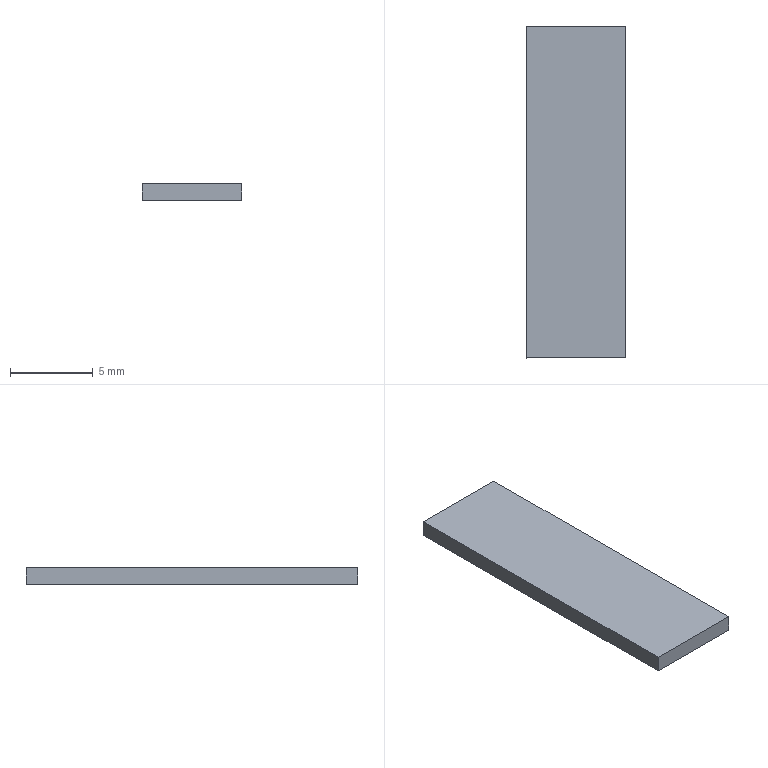Part | STEP file | RJ-USIO-V1_2-220411_235 | 1 solid | 6 faces | box 6 x 20.001 x 1 mm | volume 120.006 mm3 | plane 6
STEP:
#1=CARTESIAN_POINT('',(0.,0.,0.));
#2=DIRECTION('',(0.,0.,1.));
#3=DIRECTION('',(1.,0.,0.));
#4=AXIS2_PLACEMENT_3D('',#1,#2,#3);
#5=CARTESIAN_POINT('',(0.2,60.501,1.));
#6=VERTEX_POINT('',#5);
#7=CARTESIAN_POINT('',(0.2,40.5,1.));
#8=VERTEX_POINT('',#7);
#9=CARTESIAN_POINT('',(0.2,60.501,1.));
#10=DIRECTION('',(0.000000044,-1.,0.));
#11=VECTOR('',#10,1.);
#12=LINE('',#9,#11);
#13=CARTESIAN_POINT('',(0.2,40.5,1.));
#14=DIRECTION('',(0.,0.,-1.));
#15=DIRECTION('',(-0.000000044,1.,0.));
#16=AXIS2_PLACEMENT_3D('',#13,#14,#15);
#17=PLANE('',#16);
#18=CARTESIAN_POINT('',(20.001,0.));
#19=DIRECTION('',(-1.,0.));
#20=VECTOR('',#19,1.);
#21=LINE('',#18,#20);
#22=(GEOMETRIC_REPRESENTATION_CONTEXT(2)PARAMETRIC_REPRESENTATION_CONTEXT()REPRESENTATION_CONTEXT('',''));
#23=DEFINITIONAL_REPRESENTATION('',(#21),#22);
#24=PCURVE('',#17,#23);
#25=CARTESIAN_POINT('',(0.2,40.5,0.));
#26=DIRECTION('',(-1.,-0.000000044,0.));
#27=DIRECTION('',(0.000000044,-1.,0.));
#28=AXIS2_PLACEMENT_3D('',#25,#26,#27);
#29=PLANE('',#28);
#30=CARTESIAN_POINT('',(-20.001,1.));
#31=DIRECTION('',(1.,0.));
#32=VECTOR('',#31,1.);
#33=LINE('',#30,#32);
#34=(GEOMETRIC_REPRESENTATION_CONTEXT(2)PARAMETRIC_REPRESENTATION_CONTEXT()REPRESENTATION_CONTEXT('',''));
#35=DEFINITIONAL_REPRESENTATION('',(#33),#34);
#36=PCURVE('',#29,#35);
#37=SURFACE_CURVE('',#12,(#24,#36),.PCURVE_S1.);
#38=EDGE_CURVE('',#6,#8,#37,.T.);
#39=ORIENTED_EDGE('',*,*,#38,.T.);
#40=CARTESIAN_POINT('',(-5.8,40.5,1.));
#41=VERTEX_POINT('',#40);
#42=CARTESIAN_POINT('',(0.2,40.5,1.));
#43=DIRECTION('',(-1.,-0.000000044,0.));
#44=VECTOR('',#43,1.);
#45=LINE('',#42,#44);
#46=CARTESIAN_POINT('',(0.,0.));
#47=DIRECTION('',(0.,-1.));
#48=VECTOR('',#47,1.);
#49=LINE('',#46,#48);
#50=(GEOMETRIC_REPRESENTATION_CONTEXT(2)PARAMETRIC_REPRESENTATION_CONTEXT()REPRESENTATION_CONTEXT('',''));
#51=DEFINITIONAL_REPRESENTATION('',(#49),#50);
#52=PCURVE('',#17,#51);
#53=CARTESIAN_POINT('',(-5.8,40.5,0.));
#54=DIRECTION('',(-0.000000044,1.,0.));
#55=DIRECTION('',(-1.,-0.000000044,0.));
#56=AXIS2_PLACEMENT_3D('',#53,#54,#55);
#57=PLANE('',#56);
#58=CARTESIAN_POINT('',(-6.,1.));
#59=DIRECTION('',(1.,0.));
#60=VECTOR('',#59,1.);
#61=LINE('',#58,#60);
#62=(GEOMETRIC_REPRESENTATION_CONTEXT(2)PARAMETRIC_REPRESENTATION_CONTEXT()REPRESENTATION_CONTEXT('',''));
#63=DEFINITIONAL_REPRESENTATION('',(#61),#62);
#64=PCURVE('',#57,#63);
#65=SURFACE_CURVE('',#45,(#52,#64),.PCURVE_S1.);
#66=EDGE_CURVE('',#8,#41,#65,.T.);
#67=ORIENTED_EDGE('',*,*,#66,.T.);
#68=CARTESIAN_POINT('',(-5.8,60.501,1.));
#69=VERTEX_POINT('',#68);
#70=CARTESIAN_POINT('',(-5.8,40.5,1.));
#71=DIRECTION('',(-0.000000044,1.,0.));
#72=VECTOR('',#71,1.);
#73=LINE('',#70,#72);
#74=CARTESIAN_POINT('',(0.,-6.));
#75=DIRECTION('',(1.,0.));
#76=VECTOR('',#75,1.);
#77=LINE('',#74,#76);
#78=(GEOMETRIC_REPRESENTATION_CONTEXT(2)PARAMETRIC_REPRESENTATION_CONTEXT()REPRESENTATION_CONTEXT('',''));
#79=DEFINITIONAL_REPRESENTATION('',(#77),#78);
#80=PCURVE('',#17,#79);
#81=CARTESIAN_POINT('',(-5.8,60.5,0.));
#82=DIRECTION('',(1.,0.000000044,0.));
#83=DIRECTION('',(-0.000000044,1.,0.));
#84=AXIS2_PLACEMENT_3D('',#81,#82,#83);
#85=PLANE('',#84);
#86=CARTESIAN_POINT('',(-20.,1.));
#87=DIRECTION('',(1.,0.));
#88=VECTOR('',#87,1.);
#89=LINE('',#86,#88);
#90=(GEOMETRIC_REPRESENTATION_CONTEXT(2)PARAMETRIC_REPRESENTATION_CONTEXT()REPRESENTATION_CONTEXT('',''));
#91=DEFINITIONAL_REPRESENTATION('',(#89),#90);
#92=PCURVE('',#85,#91);
#93=SURFACE_CURVE('',#73,(#80,#92),.PCURVE_S1.);
#94=EDGE_CURVE('',#41,#69,#93,.T.);
#95=ORIENTED_EDGE('',*,*,#94,.T.);
#96=CARTESIAN_POINT('',(-5.8,60.501,1.));
#97=DIRECTION('',(1.,0.000000044,0.));
#98=VECTOR('',#97,1.);
#99=LINE('',#96,#98);
#100=CARTESIAN_POINT('',(20.001,-6.));
#101=DIRECTION('',(0.,1.));
#102=VECTOR('',#101,1.);
#103=LINE('',#100,#102);
#104=(GEOMETRIC_REPRESENTATION_CONTEXT(2)PARAMETRIC_REPRESENTATION_CONTEXT()REPRESENTATION_CONTEXT('',''));
#105=DEFINITIONAL_REPRESENTATION('',(#103),#104);
#106=PCURVE('',#17,#105);
#107=CARTESIAN_POINT('',(0.2,60.501,0.));
#108=DIRECTION('',(0.000000044,-1.,0.));
#109=DIRECTION('',(1.,0.000000044,0.));
#110=AXIS2_PLACEMENT_3D('',#107,#108,#109);
#111=PLANE('',#110);
#112=CARTESIAN_POINT('',(-6.,1.));
#113=DIRECTION('',(1.,0.));
#114=VECTOR('',#113,1.);
#115=LINE('',#112,#114);
#116=(GEOMETRIC_REPRESENTATION_CONTEXT(2)PARAMETRIC_REPRESENTATION_CONTEXT()REPRESENTATION_CONTEXT('',''));
#117=DEFINITIONAL_REPRESENTATION('',(#115),#116);
#118=PCURVE('',#111,#117);
#119=SURFACE_CURVE('',#99,(#106,#118),.PCURVE_S1.);
#120=EDGE_CURVE('',#69,#6,#119,.T.);
#121=ORIENTED_EDGE('',*,*,#120,.T.);
#122=EDGE_LOOP('',(#39,#67,#95,#121));
#123=FACE_BOUND('',#122,.F.);
#124=ADVANCED_FACE('',(#123),#17,.F.);
#125=CARTESIAN_POINT('',(0.2,60.501,0.));
#126=VERTEX_POINT('',#125);
#127=CARTESIAN_POINT('',(0.2,40.5,0.));
#128=VERTEX_POINT('',#127);
#129=CARTESIAN_POINT('',(0.2,60.501,0.));
#130=DIRECTION('',(0.000000044,-1.,0.));
#131=VECTOR('',#130,1.);
#132=LINE('',#129,#131);
#133=CARTESIAN_POINT('',(-20.001,0.));
#134=DIRECTION('',(1.,0.));
#135=VECTOR('',#134,1.);
#136=LINE('',#133,#135);
#137=(GEOMETRIC_REPRESENTATION_CONTEXT(2)PARAMETRIC_REPRESENTATION_CONTEXT()REPRESENTATION_CONTEXT('',''));
#138=DEFINITIONAL_REPRESENTATION('',(#136),#137);
#139=PCURVE('',#29,#138);
#140=CARTESIAN_POINT('',(0.2,40.5,0.));
#141=DIRECTION('',(0.,0.,-1.));
#142=DIRECTION('',(-0.000000044,1.,0.));
#143=AXIS2_PLACEMENT_3D('',#140,#141,#142);
#144=PLANE('',#143);
#145=CARTESIAN_POINT('',(20.001,0.));
#146=DIRECTION('',(-1.,0.));
#147=VECTOR('',#146,1.);
#148=LINE('',#145,#147);
#149=(GEOMETRIC_REPRESENTATION_CONTEXT(2)PARAMETRIC_REPRESENTATION_CONTEXT()REPRESENTATION_CONTEXT('',''));
#150=DEFINITIONAL_REPRESENTATION('',(#148),#149);
#151=PCURVE('',#144,#150);
#152=SURFACE_CURVE('',#132,(#139,#151),.PCURVE_S1.);
#153=EDGE_CURVE('',#126,#128,#152,.T.);
#154=ORIENTED_EDGE('',*,*,#153,.T.);
#155=CARTESIAN_POINT('',(0.2,40.5,1.));
#156=DIRECTION('',(0.,0.,-1.));
#157=VECTOR('',#156,1.);
#158=LINE('',#155,#157);
#159=CARTESIAN_POINT('',(0.,1.));
#160=DIRECTION('',(0.,-1.));
#161=VECTOR('',#160,1.);
#162=LINE('',#159,#161);
#163=(GEOMETRIC_REPRESENTATION_CONTEXT(2)PARAMETRIC_REPRESENTATION_CONTEXT()REPRESENTATION_CONTEXT('',''));
#164=DEFINITIONAL_REPRESENTATION('',(#162),#163);
#165=PCURVE('',#29,#164);
#166=CARTESIAN_POINT('',(-6.,1.));
#167=DIRECTION('',(0.,-1.));
#168=VECTOR('',#167,1.);
#169=LINE('',#166,#168);
#170=(GEOMETRIC_REPRESENTATION_CONTEXT(2)PARAMETRIC_REPRESENTATION_CONTEXT()REPRESENTATION_CONTEXT('',''));
#171=DEFINITIONAL_REPRESENTATION('',(#169),#170);
#172=PCURVE('',#57,#171);
#173=SURFACE_CURVE('',#158,(#165,#172),.PCURVE_S1.);
#174=EDGE_CURVE('',#8,#128,#173,.T.);
#175=ORIENTED_EDGE('',*,*,#174,.F.);
#176=ORIENTED_EDGE('',*,*,#38,.F.);
#177=CARTESIAN_POINT('',(0.2,60.501,1.));
#178=DIRECTION('',(0.,0.,-1.));
#179=VECTOR('',#178,1.);
#180=LINE('',#177,#179);
#181=CARTESIAN_POINT('',(-20.001,1.));
#182=DIRECTION('',(0.,-1.));
#183=VECTOR('',#182,1.);
#184=LINE('',#181,#183);
#185=(GEOMETRIC_REPRESENTATION_CONTEXT(2)PARAMETRIC_REPRESENTATION_CONTEXT()REPRESENTATION_CONTEXT('',''));
#186=DEFINITIONAL_REPRESENTATION('',(#184),#185);
#187=PCURVE('',#29,#186);
#188=CARTESIAN_POINT('',(0.,1.));
#189=DIRECTION('',(0.,-1.));
#190=VECTOR('',#189,1.);
#191=LINE('',#188,#190);
#192=(GEOMETRIC_REPRESENTATION_CONTEXT(2)PARAMETRIC_REPRESENTATION_CONTEXT()REPRESENTATION_CONTEXT('',''));
#193=DEFINITIONAL_REPRESENTATION('',(#191),#192);
#194=PCURVE('',#111,#193);
#195=SURFACE_CURVE('',#180,(#187,#194),.PCURVE_S1.);
#196=EDGE_CURVE('',#6,#126,#195,.T.);
#197=ORIENTED_EDGE('',*,*,#196,.T.);
#198=EDGE_LOOP('',(#154,#175,#176,#197));
#199=FACE_BOUND('',#198,.F.);
#200=ADVANCED_FACE('',(#199),#29,.F.);
#201=CARTESIAN_POINT('',(-5.8,40.5,0.));
#202=VERTEX_POINT('',#201);
#203=CARTESIAN_POINT('',(0.2,40.5,0.));
#204=DIRECTION('',(-1.,-0.000000044,0.));
#205=VECTOR('',#204,1.);
#206=LINE('',#203,#205);
#207=CARTESIAN_POINT('',(0.,0.));
#208=DIRECTION('',(0.,-1.));
#209=VECTOR('',#208,1.);
#210=LINE('',#207,#209);
#211=(GEOMETRIC_REPRESENTATION_CONTEXT(2)PARAMETRIC_REPRESENTATION_CONTEXT()REPRESENTATION_CONTEXT('',''));
#212=DEFINITIONAL_REPRESENTATION('',(#210),#211);
#213=PCURVE('',#144,#212);
#214=CARTESIAN_POINT('',(-6.,0.));
#215=DIRECTION('',(1.,0.));
#216=VECTOR('',#215,1.);
#217=LINE('',#214,#216);
#218=(GEOMETRIC_REPRESENTATION_CONTEXT(2)PARAMETRIC_REPRESENTATION_CONTEXT()REPRESENTATION_CONTEXT('',''));
#219=DEFINITIONAL_REPRESENTATION('',(#217),#218);
#220=PCURVE('',#57,#219);
#221=SURFACE_CURVE('',#206,(#213,#220),.PCURVE_S1.);
#222=EDGE_CURVE('',#128,#202,#221,.T.);
#223=ORIENTED_EDGE('',*,*,#222,.F.);
#224=ORIENTED_EDGE('',*,*,#153,.F.);
#225=CARTESIAN_POINT('',(-5.8,60.501,0.));
#226=VERTEX_POINT('',#225);
#227=CARTESIAN_POINT('',(-5.8,60.501,0.));
#228=DIRECTION('',(1.,0.000000044,0.));
#229=VECTOR('',#228,1.);
#230=LINE('',#227,#229);
#231=CARTESIAN_POINT('',(20.001,-6.));
#232=DIRECTION('',(0.,1.));
#233=VECTOR('',#232,1.);
#234=LINE('',#231,#233);
#235=(GEOMETRIC_REPRESENTATION_CONTEXT(2)PARAMETRIC_REPRESENTATION_CONTEXT()REPRESENTATION_CONTEXT('',''));
#236=DEFINITIONAL_REPRESENTATION('',(#234),#235);
#237=PCURVE('',#144,#236);
#238=CARTESIAN_POINT('',(-6.,0.));
#239=DIRECTION('',(1.,0.));
#240=VECTOR('',#239,1.);
#241=LINE('',#238,#240);
#242=(GEOMETRIC_REPRESENTATION_CONTEXT(2)PARAMETRIC_REPRESENTATION_CONTEXT()REPRESENTATION_CONTEXT('',''));
#243=DEFINITIONAL_REPRESENTATION('',(#241),#242);
#244=PCURVE('',#111,#243);
#245=SURFACE_CURVE('',#230,(#237,#244),.PCURVE_S1.);
#246=EDGE_CURVE('',#226,#126,#245,.T.);
#247=ORIENTED_EDGE('',*,*,#246,.F.);
#248=CARTESIAN_POINT('',(-5.8,40.5,0.));
#249=DIRECTION('',(-0.000000044,1.,0.));
#250=VECTOR('',#249,1.);
#251=LINE('',#248,#250);
#252=CARTESIAN_POINT('',(0.,-6.));
#253=DIRECTION('',(1.,0.));
#254=VECTOR('',#253,1.);
#255=LINE('',#252,#254);
#256=(GEOMETRIC_REPRESENTATION_CONTEXT(2)PARAMETRIC_REPRESENTATION_CONTEXT()REPRESENTATION_CONTEXT('',''));
#257=DEFINITIONAL_REPRESENTATION('',(#255),#256);
#258=PCURVE('',#144,#257);
#259=CARTESIAN_POINT('',(-20.,0.));
#260=DIRECTION('',(1.,0.));
#261=VECTOR('',#260,1.);
#262=LINE('',#259,#261);
#263=(GEOMETRIC_REPRESENTATION_CONTEXT(2)PARAMETRIC_REPRESENTATION_CONTEXT()REPRESENTATION_CONTEXT('',''));
#264=DEFINITIONAL_REPRESENTATION('',(#262),#263);
#265=PCURVE('',#85,#264);
#266=SURFACE_CURVE('',#251,(#258,#265),.PCURVE_S1.);
#267=EDGE_CURVE('',#202,#226,#266,.T.);
#268=ORIENTED_EDGE('',*,*,#267,.F.);
#269=EDGE_LOOP('',(#223,#224,#247,#268));
#270=FACE_BOUND('',#269,.F.);
#271=ADVANCED_FACE('',(#270),#144,.T.);
#272=ORIENTED_EDGE('',*,*,#222,.T.);
#273=CARTESIAN_POINT('',(-5.8,40.5,1.));
#274=DIRECTION('',(0.,0.,-1.));
#275=VECTOR('',#274,1.);
#276=LINE('',#273,#275);
#277=CARTESIAN_POINT('',(0.,1.));
#278=DIRECTION('',(0.,-1.));
#279=VECTOR('',#278,1.);
#280=LINE('',#277,#279);
#281=(GEOMETRIC_REPRESENTATION_CONTEXT(2)PARAMETRIC_REPRESENTATION_CONTEXT()REPRESENTATION_CONTEXT('',''));
#282=DEFINITIONAL_REPRESENTATION('',(#280),#281);
#283=PCURVE('',#57,#282);
#284=CARTESIAN_POINT('',(-20.,1.));
#285=DIRECTION('',(0.,-1.));
#286=VECTOR('',#285,1.);
#287=LINE('',#284,#286);
#288=(GEOMETRIC_REPRESENTATION_CONTEXT(2)PARAMETRIC_REPRESENTATION_CONTEXT()REPRESENTATION_CONTEXT('',''));
#289=DEFINITIONAL_REPRESENTATION('',(#287),#288);
#290=PCURVE('',#85,#289);
#291=SURFACE_CURVE('',#276,(#283,#290),.PCURVE_S1.);
#292=EDGE_CURVE('',#41,#202,#291,.T.);
#293=ORIENTED_EDGE('',*,*,#292,.F.);
#294=ORIENTED_EDGE('',*,*,#66,.F.);
#295=ORIENTED_EDGE('',*,*,#174,.T.);
#296=EDGE_LOOP('',(#272,#293,#294,#295));
#297=FACE_BOUND('',#296,.F.);
#298=ADVANCED_FACE('',(#297),#57,.F.);
#299=ORIENTED_EDGE('',*,*,#267,.T.);
#300=CARTESIAN_POINT('',(-5.8,60.501,1.));
#301=DIRECTION('',(0.,0.,-1.));
#302=VECTOR('',#301,1.);
#303=LINE('',#300,#302);
#304=CARTESIAN_POINT('',(0.001001,1.));
#305=DIRECTION('',(0.,-1.));
#306=VECTOR('',#305,1.);
#307=LINE('',#304,#306);
#308=(GEOMETRIC_REPRESENTATION_CONTEXT(2)PARAMETRIC_REPRESENTATION_CONTEXT()REPRESENTATION_CONTEXT('',''));
#309=DEFINITIONAL_REPRESENTATION('',(#307),#308);
#310=PCURVE('',#85,#309);
#311=CARTESIAN_POINT('',(-6.,1.));
#312=DIRECTION('',(0.,-1.));
#313=VECTOR('',#312,1.);
#314=LINE('',#311,#313);
#315=(GEOMETRIC_REPRESENTATION_CONTEXT(2)PARAMETRIC_REPRESENTATION_CONTEXT()REPRESENTATION_CONTEXT('',''));
#316=DEFINITIONAL_REPRESENTATION('',(#314),#315);
#317=PCURVE('',#111,#316);
#318=SURFACE_CURVE('',#303,(#310,#317),.PCURVE_S1.);
#319=EDGE_CURVE('',#69,#226,#318,.T.);
#320=ORIENTED_EDGE('',*,*,#319,.F.);
#321=ORIENTED_EDGE('',*,*,#94,.F.);
#322=ORIENTED_EDGE('',*,*,#292,.T.);
#323=EDGE_LOOP('',(#299,#320,#321,#322));
#324=FACE_BOUND('',#323,.F.);
#325=ADVANCED_FACE('',(#324),#85,.F.);
#326=ORIENTED_EDGE('',*,*,#246,.T.);
#327=ORIENTED_EDGE('',*,*,#196,.F.);
#328=ORIENTED_EDGE('',*,*,#120,.F.);
#329=ORIENTED_EDGE('',*,*,#319,.T.);
#330=EDGE_LOOP('',(#326,#327,#328,#329));
#331=FACE_BOUND('',#330,.F.);
#332=ADVANCED_FACE('',(#331),#111,.F.);
#333=CLOSED_SHELL('',(#124,#200,#271,#298,#325,#332));
#334=MANIFOLD_SOLID_BREP('',#333);
#335=(LENGTH_UNIT()NAMED_UNIT(*)SI_UNIT(.MILLI.,.METRE.));
#336=UNCERTAINTY_MEASURE_WITH_UNIT(LENGTH_MEASURE(0.0000001),#335,'','');
#337=(NAMED_UNIT(*)PLANE_ANGLE_UNIT()SI_UNIT($,.RADIAN.));
#338=(NAMED_UNIT(*)SI_UNIT($,.STERADIAN.)SOLID_ANGLE_UNIT());
#339=(GEOMETRIC_REPRESENTATION_CONTEXT(3)GLOBAL_UNCERTAINTY_ASSIGNED_CONTEXT((#336))GLOBAL_UNIT_ASSIGNED_CONTEXT((#335,#337,#338))REPRESENTATION_CONTEXT('',''));
#340=ADVANCED_BREP_SHAPE_REPRESENTATION('',(#4,#334),#339);